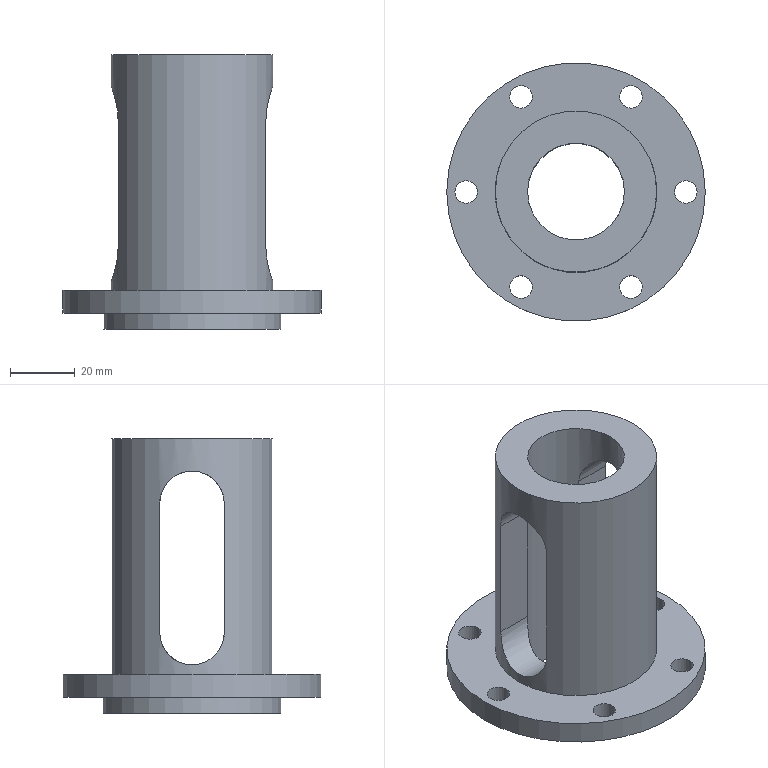Part | NX | 1 solid | 22 faces | box 80 x 80 x 85 mm | volume 105355 mm3 | cylinder 14 | plane 8 | commonest cylinder face diameters 7 x6 20 x4 30 x1 50 x1 55 x1 80 x1
STEP:
#1=CARTESIAN_POINT('',(-18.75,-32.476,12.));
#2=VERTEX_POINT('',#1);
#3=CARTESIAN_POINT('',(-17.,-29.445,12.));
#4=DIRECTION('',(0.,0.,1.));
#5=DIRECTION('',(-0.5,-0.866,0.));
#6=AXIS2_PLACEMENT_3D('',#3,#4,#5);
#7=CIRCLE('',#6,3.5);
#8=EDGE_CURVE('',#2,#2,#7,.T.);
#9=ORIENTED_EDGE('',*,*,#8,.T.);
#10=EDGE_LOOP('',(#9));
#11=FACE_BOUND('',#10,.T.);
#12=CARTESIAN_POINT('',(-18.75,-32.476,5.));
#13=VERTEX_POINT('',#12);
#14=CARTESIAN_POINT('',(-17.,-29.445,5.));
#15=DIRECTION('',(0.,0.,1.));
#16=DIRECTION('',(-0.5,-0.866,0.));
#17=AXIS2_PLACEMENT_3D('',#14,#15,#16);
#18=CIRCLE('',#17,3.5);
#19=EDGE_CURVE('',#13,#13,#18,.T.);
#20=ORIENTED_EDGE('',*,*,#19,.F.);
#21=EDGE_LOOP('',(#20));
#22=FACE_BOUND('',#21,.T.);
#23=CARTESIAN_POINT('',(-17.,-29.445,12.));
#24=DIRECTION('',(0.,0.,-1.));
#25=DIRECTION('',(-1.,0.,0.));
#26=AXIS2_PLACEMENT_3D('',#23,#24,#25);
#27=CYLINDRICAL_SURFACE('',#26,3.5);
#28=ADVANCED_FACE('',(#11,#22),#27,.F.);
#29=CARTESIAN_POINT('',(-18.75,32.476,12.));
#30=VERTEX_POINT('',#29);
#31=CARTESIAN_POINT('',(-17.,29.445,12.));
#32=DIRECTION('',(0.,0.,1.));
#33=DIRECTION('',(-0.5,0.866,0.));
#34=AXIS2_PLACEMENT_3D('',#31,#32,#33);
#35=CIRCLE('',#34,3.5);
#36=EDGE_CURVE('',#30,#30,#35,.T.);
#37=ORIENTED_EDGE('',*,*,#36,.T.);
#38=EDGE_LOOP('',(#37));
#39=FACE_BOUND('',#38,.T.);
#40=CARTESIAN_POINT('',(-18.75,32.476,5.));
#41=VERTEX_POINT('',#40);
#42=CARTESIAN_POINT('',(-17.,29.445,5.));
#43=DIRECTION('',(0.,0.,1.));
#44=DIRECTION('',(-0.5,0.866,0.));
#45=AXIS2_PLACEMENT_3D('',#42,#43,#44);
#46=CIRCLE('',#45,3.5);
#47=EDGE_CURVE('',#41,#41,#46,.T.);
#48=ORIENTED_EDGE('',*,*,#47,.F.);
#49=EDGE_LOOP('',(#48));
#50=FACE_BOUND('',#49,.T.);
#51=CARTESIAN_POINT('',(-17.,29.445,12.));
#52=DIRECTION('',(0.,0.,-1.));
#53=DIRECTION('',(-1.,0.,0.));
#54=AXIS2_PLACEMENT_3D('',#51,#52,#53);
#55=CYLINDRICAL_SURFACE('',#54,3.5);
#56=ADVANCED_FACE('',(#39,#50),#55,.F.);
#57=CARTESIAN_POINT('',(18.75,-32.476,12.));
#58=VERTEX_POINT('',#57);
#59=CARTESIAN_POINT('',(17.,-29.445,12.));
#60=DIRECTION('',(0.,0.,1.));
#61=DIRECTION('',(0.5,-0.866,0.));
#62=AXIS2_PLACEMENT_3D('',#59,#60,#61);
#63=CIRCLE('',#62,3.5);
#64=EDGE_CURVE('',#58,#58,#63,.T.);
#65=ORIENTED_EDGE('',*,*,#64,.T.);
#66=EDGE_LOOP('',(#65));
#67=FACE_BOUND('',#66,.T.);
#68=CARTESIAN_POINT('',(18.75,-32.476,5.));
#69=VERTEX_POINT('',#68);
#70=CARTESIAN_POINT('',(17.,-29.445,5.));
#71=DIRECTION('',(0.,0.,1.));
#72=DIRECTION('',(0.5,-0.866,0.));
#73=AXIS2_PLACEMENT_3D('',#70,#71,#72);
#74=CIRCLE('',#73,3.5);
#75=EDGE_CURVE('',#69,#69,#74,.T.);
#76=ORIENTED_EDGE('',*,*,#75,.F.);
#77=EDGE_LOOP('',(#76));
#78=FACE_BOUND('',#77,.T.);
#79=CARTESIAN_POINT('',(17.,-29.445,12.));
#80=DIRECTION('',(0.,0.,-1.));
#81=DIRECTION('',(-1.,0.,0.));
#82=AXIS2_PLACEMENT_3D('',#79,#80,#81);
#83=CYLINDRICAL_SURFACE('',#82,3.5);
#84=ADVANCED_FACE('',(#67,#78),#83,.F.);
#85=CARTESIAN_POINT('',(18.75,32.476,12.));
#86=VERTEX_POINT('',#85);
#87=CARTESIAN_POINT('',(17.,29.445,12.));
#88=DIRECTION('',(0.,0.,1.));
#89=DIRECTION('',(0.5,0.866,0.));
#90=AXIS2_PLACEMENT_3D('',#87,#88,#89);
#91=CIRCLE('',#90,3.5);
#92=EDGE_CURVE('',#86,#86,#91,.T.);
#93=ORIENTED_EDGE('',*,*,#92,.T.);
#94=EDGE_LOOP('',(#93));
#95=FACE_BOUND('',#94,.T.);
#96=CARTESIAN_POINT('',(18.75,32.476,5.));
#97=VERTEX_POINT('',#96);
#98=CARTESIAN_POINT('',(17.,29.445,5.));
#99=DIRECTION('',(0.,0.,1.));
#100=DIRECTION('',(0.5,0.866,0.));
#101=AXIS2_PLACEMENT_3D('',#98,#99,#100);
#102=CIRCLE('',#101,3.5);
#103=EDGE_CURVE('',#97,#97,#102,.T.);
#104=ORIENTED_EDGE('',*,*,#103,.F.);
#105=EDGE_LOOP('',(#104));
#106=FACE_BOUND('',#105,.T.);
#107=CARTESIAN_POINT('',(17.,29.445,12.));
#108=DIRECTION('',(0.,0.,-1.));
#109=DIRECTION('',(-1.,0.,0.));
#110=AXIS2_PLACEMENT_3D('',#107,#108,#109);
#111=CYLINDRICAL_SURFACE('',#110,3.5);
#112=ADVANCED_FACE('',(#95,#106),#111,.F.);
#113=CARTESIAN_POINT('',(37.5,0.,12.));
#114=VERTEX_POINT('',#113);
#115=CARTESIAN_POINT('',(34.,0.,12.));
#116=DIRECTION('',(0.,0.,1.));
#117=DIRECTION('',(1.,0.,0.));
#118=AXIS2_PLACEMENT_3D('',#115,#116,#117);
#119=CIRCLE('',#118,3.5);
#120=EDGE_CURVE('',#114,#114,#119,.T.);
#121=ORIENTED_EDGE('',*,*,#120,.T.);
#122=EDGE_LOOP('',(#121));
#123=FACE_BOUND('',#122,.T.);
#124=CARTESIAN_POINT('',(37.5,0.,5.));
#125=VERTEX_POINT('',#124);
#126=CARTESIAN_POINT('',(34.,0.,5.));
#127=DIRECTION('',(0.,0.,1.));
#128=DIRECTION('',(1.,0.,0.));
#129=AXIS2_PLACEMENT_3D('',#126,#127,#128);
#130=CIRCLE('',#129,3.5);
#131=EDGE_CURVE('',#125,#125,#130,.T.);
#132=ORIENTED_EDGE('',*,*,#131,.F.);
#133=EDGE_LOOP('',(#132));
#134=FACE_BOUND('',#133,.T.);
#135=CARTESIAN_POINT('',(34.,0.,12.));
#136=DIRECTION('',(0.,0.,-1.));
#137=DIRECTION('',(-1.,0.,0.));
#138=AXIS2_PLACEMENT_3D('',#135,#136,#137);
#139=CYLINDRICAL_SURFACE('',#138,3.5);
#140=ADVANCED_FACE('',(#123,#134),#139,.F.);
#141=CARTESIAN_POINT('',(40.,0.,12.));
#142=VERTEX_POINT('',#141);
#143=CARTESIAN_POINT('',(0.,0.,12.));
#144=DIRECTION('',(0.,0.,1.));
#145=DIRECTION('',(1.,0.,0.));
#146=AXIS2_PLACEMENT_3D('',#143,#144,#145);
#147=CIRCLE('',#146,40.);
#148=EDGE_CURVE('',#142,#142,#147,.T.);
#149=ORIENTED_EDGE('',*,*,#148,.F.);
#150=EDGE_LOOP('',(#149));
#151=FACE_BOUND('',#150,.T.);
#152=CARTESIAN_POINT('',(40.,0.,5.));
#153=VERTEX_POINT('',#152);
#154=CARTESIAN_POINT('',(0.,0.,5.));
#155=DIRECTION('',(0.,0.,-1.));
#156=DIRECTION('',(1.,0.,0.));
#157=AXIS2_PLACEMENT_3D('',#154,#155,#156);
#158=CIRCLE('',#157,40.);
#159=EDGE_CURVE('',#153,#153,#158,.T.);
#160=ORIENTED_EDGE('',*,*,#159,.F.);
#161=EDGE_LOOP('',(#160));
#162=FACE_BOUND('',#161,.T.);
#163=CARTESIAN_POINT('',(0.,0.,12.));
#164=DIRECTION('',(0.,0.,-1.));
#165=DIRECTION('',(-1.,0.,0.));
#166=AXIS2_PLACEMENT_3D('',#163,#164,#165);
#167=CYLINDRICAL_SURFACE('',#166,40.);
#168=ADVANCED_FACE('',(#151,#162),#167,.T.);
#169=CARTESIAN_POINT('',(-37.5,0.,12.));
#170=VERTEX_POINT('',#169);
#171=CARTESIAN_POINT('',(-34.,0.,12.));
#172=DIRECTION('',(0.,0.,1.));
#173=DIRECTION('',(-1.,0.,0.));
#174=AXIS2_PLACEMENT_3D('',#171,#172,#173);
#175=CIRCLE('',#174,3.5);
#176=EDGE_CURVE('',#170,#170,#175,.T.);
#177=ORIENTED_EDGE('',*,*,#176,.T.);
#178=EDGE_LOOP('',(#177));
#179=FACE_BOUND('',#178,.T.);
#180=CARTESIAN_POINT('',(-37.5,0.,5.));
#181=VERTEX_POINT('',#180);
#182=CARTESIAN_POINT('',(-34.,0.,5.));
#183=DIRECTION('',(0.,0.,1.));
#184=DIRECTION('',(-1.,0.,0.));
#185=AXIS2_PLACEMENT_3D('',#182,#183,#184);
#186=CIRCLE('',#185,3.5);
#187=EDGE_CURVE('',#181,#181,#186,.T.);
#188=ORIENTED_EDGE('',*,*,#187,.F.);
#189=EDGE_LOOP('',(#188));
#190=FACE_BOUND('',#189,.T.);
#191=CARTESIAN_POINT('',(-34.,0.,12.));
#192=DIRECTION('',(0.,0.,-1.));
#193=DIRECTION('',(-1.,0.,0.));
#194=AXIS2_PLACEMENT_3D('',#191,#192,#193);
#195=CYLINDRICAL_SURFACE('',#194,3.5);
#196=ADVANCED_FACE('',(#179,#190),#195,.F.);
#197=CARTESIAN_POINT('',(22.913,10.,65.));
#198=VERTEX_POINT('',#197);
#199=CARTESIAN_POINT('',(22.913,-10.,65.));
#200=VERTEX_POINT('',#199);
#201=CARTESIAN_POINT('',(22.913,10.,65.));
#202=CARTESIAN_POINT('',(22.913,10.,67.672));
#203=CARTESIAN_POINT('',(23.712,8.35,71.514));
#204=CARTESIAN_POINT('',(24.779,3.969,74.459));
#205=CARTESIAN_POINT('',(25.11,0.01559,75.268));
#206=CARTESIAN_POINT('',(24.782,-3.957,74.467));
#207=CARTESIAN_POINT('',(23.711,-8.353,71.514));
#208=CARTESIAN_POINT('',(22.913,-10.,67.673));
#209=CARTESIAN_POINT('',(22.913,-10.,65.));
#210=B_SPLINE_CURVE_WITH_KNOTS('',3,(#201,#202,#203,#204,#205,#206,#207,#208,#209),.UNSPECIFIED.,.F.,.F.,(4,1,1,1,1,1,4),(0.,0.007896,0.01184,0.01579,0.01974,0.02369,0.03158),.UNSPECIFIED.);
#211=EDGE_CURVE('',#198,#200,#210,.T.);
#212=ORIENTED_EDGE('',*,*,#211,.F.);
#213=CARTESIAN_POINT('',(22.913,10.,25.));
#214=VERTEX_POINT('',#213);
#215=CARTESIAN_POINT('',(22.913,10.,85.));
#216=DIRECTION('',(0.,0.,-1.));
#217=VECTOR('',#216,1000.);
#218=LINE('',#215,#217);
#219=EDGE_CURVE('',#214,#198,#218,.F.);
#220=ORIENTED_EDGE('',*,*,#219,.F.);
#221=CARTESIAN_POINT('',(22.913,-10.,25.));
#222=VERTEX_POINT('',#221);
#223=CARTESIAN_POINT('',(22.913,-10.,25.));
#224=CARTESIAN_POINT('',(22.913,-10.,22.328));
#225=CARTESIAN_POINT('',(23.712,-8.35,18.486));
#226=CARTESIAN_POINT('',(24.779,-3.969,15.541));
#227=CARTESIAN_POINT('',(25.11,-0.01559,14.732));
#228=CARTESIAN_POINT('',(24.782,3.957,15.533));
#229=CARTESIAN_POINT('',(23.711,8.353,18.486));
#230=CARTESIAN_POINT('',(22.913,10.,22.327));
#231=CARTESIAN_POINT('',(22.913,10.,25.));
#232=B_SPLINE_CURVE_WITH_KNOTS('',3,(#223,#224,#225,#226,#227,#228,#229,#230,#231),.UNSPECIFIED.,.F.,.F.,(4,1,1,1,1,1,4),(0.,0.007896,0.01184,0.01579,0.01974,0.02369,0.03158),.UNSPECIFIED.);
#233=EDGE_CURVE('',#222,#214,#232,.T.);
#234=ORIENTED_EDGE('',*,*,#233,.F.);
#235=CARTESIAN_POINT('',(22.913,-10.,85.));
#236=DIRECTION('',(0.,0.,-1.));
#237=VECTOR('',#236,1000.);
#238=LINE('',#235,#237);
#239=EDGE_CURVE('',#200,#222,#238,.T.);
#240=ORIENTED_EDGE('',*,*,#239,.F.);
#241=EDGE_LOOP('',(#212,#220,#234,#240));
#242=FACE_BOUND('',#241,.T.);
#243=CARTESIAN_POINT('',(25.,0.,85.));
#244=VERTEX_POINT('',#243);
#245=CARTESIAN_POINT('',(0.,0.,85.));
#246=DIRECTION('',(0.,0.,1.));
#247=DIRECTION('',(1.,0.,0.));
#248=AXIS2_PLACEMENT_3D('',#245,#246,#247);
#249=CIRCLE('',#248,25.);
#250=EDGE_CURVE('',#244,#244,#249,.T.);
#251=ORIENTED_EDGE('',*,*,#250,.F.);
#252=EDGE_LOOP('',(#251));
#253=FACE_BOUND('',#252,.T.);
#254=CARTESIAN_POINT('',(25.,0.,12.));
#255=VERTEX_POINT('',#254);
#256=CARTESIAN_POINT('',(0.,0.,12.));
#257=DIRECTION('',(0.,0.,1.));
#258=DIRECTION('',(1.,0.,0.));
#259=AXIS2_PLACEMENT_3D('',#256,#257,#258);
#260=CIRCLE('',#259,25.);
#261=EDGE_CURVE('',#255,#255,#260,.T.);
#262=ORIENTED_EDGE('',*,*,#261,.T.);
#263=EDGE_LOOP('',(#262));
#264=FACE_BOUND('',#263,.T.);
#265=CARTESIAN_POINT('',(-22.913,10.,65.));
#266=VERTEX_POINT('',#265);
#267=CARTESIAN_POINT('',(-22.913,10.,25.));
#268=VERTEX_POINT('',#267);
#269=CARTESIAN_POINT('',(-22.913,10.,85.));
#270=DIRECTION('',(0.,0.,-1.));
#271=VECTOR('',#270,1000.);
#272=LINE('',#269,#271);
#273=EDGE_CURVE('',#266,#268,#272,.T.);
#274=ORIENTED_EDGE('',*,*,#273,.F.);
#275=CARTESIAN_POINT('',(-22.913,-10.,65.));
#276=VERTEX_POINT('',#275);
#277=CARTESIAN_POINT('',(-22.913,-10.,65.));
#278=CARTESIAN_POINT('',(-22.913,-10.,67.672));
#279=CARTESIAN_POINT('',(-23.712,-8.35,71.514));
#280=CARTESIAN_POINT('',(-24.779,-3.969,74.459));
#281=CARTESIAN_POINT('',(-25.11,-0.01559,75.268));
#282=CARTESIAN_POINT('',(-24.782,3.957,74.467));
#283=CARTESIAN_POINT('',(-23.711,8.353,71.514));
#284=CARTESIAN_POINT('',(-22.913,10.,67.673));
#285=CARTESIAN_POINT('',(-22.913,10.,65.));
#286=B_SPLINE_CURVE_WITH_KNOTS('',3,(#277,#278,#279,#280,#281,#282,#283,#284,#285),.UNSPECIFIED.,.F.,.F.,(4,1,1,1,1,1,4),(0.,0.007896,0.01184,0.01579,0.01974,0.02369,0.03158),.UNSPECIFIED.);
#287=EDGE_CURVE('',#276,#266,#286,.T.);
#288=ORIENTED_EDGE('',*,*,#287,.F.);
#289=CARTESIAN_POINT('',(-22.913,-10.,25.));
#290=VERTEX_POINT('',#289);
#291=CARTESIAN_POINT('',(-22.913,-10.,85.));
#292=DIRECTION('',(0.,0.,-1.));
#293=VECTOR('',#292,1000.);
#294=LINE('',#291,#293);
#295=EDGE_CURVE('',#290,#276,#294,.F.);
#296=ORIENTED_EDGE('',*,*,#295,.F.);
#297=CARTESIAN_POINT('',(-22.913,10.,25.));
#298=CARTESIAN_POINT('',(-22.913,10.,22.328));
#299=CARTESIAN_POINT('',(-23.712,8.35,18.486));
#300=CARTESIAN_POINT('',(-24.779,3.969,15.541));
#301=CARTESIAN_POINT('',(-25.11,0.01559,14.732));
#302=CARTESIAN_POINT('',(-24.782,-3.957,15.533));
#303=CARTESIAN_POINT('',(-23.711,-8.353,18.486));
#304=CARTESIAN_POINT('',(-22.913,-10.,22.327));
#305=CARTESIAN_POINT('',(-22.913,-10.,25.));
#306=B_SPLINE_CURVE_WITH_KNOTS('',3,(#297,#298,#299,#300,#301,#302,#303,#304,#305),.UNSPECIFIED.,.F.,.F.,(4,1,1,1,1,1,4),(0.,0.007896,0.01184,0.01579,0.01974,0.02369,0.03158),.UNSPECIFIED.);
#307=EDGE_CURVE('',#268,#290,#306,.T.);
#308=ORIENTED_EDGE('',*,*,#307,.F.);
#309=EDGE_LOOP('',(#274,#288,#296,#308));
#310=FACE_BOUND('',#309,.T.);
#311=CARTESIAN_POINT('',(0.,0.,85.));
#312=DIRECTION('',(0.,0.,-1.));
#313=DIRECTION('',(-1.,0.,0.));
#314=AXIS2_PLACEMENT_3D('',#311,#312,#313);
#315=CYLINDRICAL_SURFACE('',#314,25.);
#316=ADVANCED_FACE('',(#242,#253,#264,#310),#315,.T.);
#317=CARTESIAN_POINT('',(15.,0.,85.));
#318=VERTEX_POINT('',#317);
#319=CARTESIAN_POINT('',(0.,0.,85.));
#320=DIRECTION('',(0.,0.,1.));
#321=DIRECTION('',(1.,0.,0.));
#322=AXIS2_PLACEMENT_3D('',#319,#320,#321);
#323=CIRCLE('',#322,15.);
#324=EDGE_CURVE('',#318,#318,#323,.T.);
#325=ORIENTED_EDGE('',*,*,#324,.T.);
#326=EDGE_LOOP('',(#325));
#327=FACE_BOUND('',#326,.T.);
#328=CARTESIAN_POINT('',(15.,0.,0.));
#329=VERTEX_POINT('',#328);
#330=CARTESIAN_POINT('',(0.,0.,0.));
#331=DIRECTION('',(0.,0.,1.));
#332=DIRECTION('',(1.,0.,0.));
#333=AXIS2_PLACEMENT_3D('',#330,#331,#332);
#334=CIRCLE('',#333,15.);
#335=EDGE_CURVE('',#329,#329,#334,.T.);
#336=ORIENTED_EDGE('',*,*,#335,.F.);
#337=EDGE_LOOP('',(#336));
#338=FACE_BOUND('',#337,.T.);
#339=CARTESIAN_POINT('',(11.18,-10.,25.));
#340=VERTEX_POINT('',#339);
#341=CARTESIAN_POINT('',(11.18,10.,25.));
#342=VERTEX_POINT('',#341);
#343=CARTESIAN_POINT('',(11.18,-10.,25.));
#344=CARTESIAN_POINT('',(11.18,-10.,23.63));
#345=CARTESIAN_POINT('',(11.718,-9.43,20.978));
#346=CARTESIAN_POINT('',(13.243,-7.268,17.79));
#347=CARTESIAN_POINT('',(14.604,-4.071,15.581));
#348=CARTESIAN_POINT('',(15.195,-0.03414,14.714));
#349=CARTESIAN_POINT('',(14.616,4.041,15.562));
#350=CARTESIAN_POINT('',(13.247,7.261,17.785));
#351=CARTESIAN_POINT('',(11.727,9.419,20.951));
#352=CARTESIAN_POINT('',(11.18,10.,23.627));
#353=CARTESIAN_POINT('',(11.18,10.,25.));
#354=B_SPLINE_CURVE_WITH_KNOTS('',3,(#343,#344,#345,#346,#347,#348,#349,#350,#351,#352,#353),.UNSPECIFIED.,.F.,.F.,(4,1,1,1,1,1,1,1,4),(0.,0.004037,0.008074,0.01211,0.01615,0.02018,0.02422,0.02826,0.0323),.UNSPECIFIED.);
#355=EDGE_CURVE('',#340,#342,#354,.T.);
#356=ORIENTED_EDGE('',*,*,#355,.T.);
#357=CARTESIAN_POINT('',(11.18,10.,65.));
#358=VERTEX_POINT('',#357);
#359=CARTESIAN_POINT('',(11.18,10.,85.));
#360=DIRECTION('',(0.,0.,-1.));
#361=VECTOR('',#360,1000.);
#362=LINE('',#359,#361);
#363=EDGE_CURVE('',#342,#358,#362,.F.);
#364=ORIENTED_EDGE('',*,*,#363,.T.);
#365=CARTESIAN_POINT('',(11.18,-10.,65.));
#366=VERTEX_POINT('',#365);
#367=CARTESIAN_POINT('',(11.18,10.,65.));
#368=CARTESIAN_POINT('',(11.18,10.,66.37));
#369=CARTESIAN_POINT('',(11.718,9.43,69.022));
#370=CARTESIAN_POINT('',(13.243,7.268,72.21));
#371=CARTESIAN_POINT('',(14.604,4.071,74.419));
#372=CARTESIAN_POINT('',(15.195,0.03414,75.286));
#373=CARTESIAN_POINT('',(14.616,-4.041,74.438));
#374=CARTESIAN_POINT('',(13.247,-7.261,72.215));
#375=CARTESIAN_POINT('',(11.727,-9.419,69.049));
#376=CARTESIAN_POINT('',(11.18,-10.,66.373));
#377=CARTESIAN_POINT('',(11.18,-10.,65.));
#378=B_SPLINE_CURVE_WITH_KNOTS('',3,(#367,#368,#369,#370,#371,#372,#373,#374,#375,#376,#377),.UNSPECIFIED.,.F.,.F.,(4,1,1,1,1,1,1,1,4),(0.,0.004037,0.008074,0.01211,0.01615,0.02018,0.02422,0.02826,0.0323),.UNSPECIFIED.);
#379=EDGE_CURVE('',#358,#366,#378,.T.);
#380=ORIENTED_EDGE('',*,*,#379,.T.);
#381=CARTESIAN_POINT('',(11.18,-10.,85.));
#382=DIRECTION('',(0.,0.,-1.));
#383=VECTOR('',#382,1000.);
#384=LINE('',#381,#383);
#385=EDGE_CURVE('',#366,#340,#384,.T.);
#386=ORIENTED_EDGE('',*,*,#385,.T.);
#387=EDGE_LOOP('',(#356,#364,#380,#386));
#388=FACE_BOUND('',#387,.T.);
#389=CARTESIAN_POINT('',(-11.18,-10.,65.));
#390=VERTEX_POINT('',#389);
#391=CARTESIAN_POINT('',(-11.18,10.,65.));
#392=VERTEX_POINT('',#391);
#393=CARTESIAN_POINT('',(-11.18,-10.,65.));
#394=CARTESIAN_POINT('',(-11.18,-10.,66.37));
#395=CARTESIAN_POINT('',(-11.718,-9.43,69.022));
#396=CARTESIAN_POINT('',(-13.243,-7.268,72.21));
#397=CARTESIAN_POINT('',(-14.604,-4.071,74.419));
#398=CARTESIAN_POINT('',(-15.195,-0.03414,75.286));
#399=CARTESIAN_POINT('',(-14.616,4.041,74.438));
#400=CARTESIAN_POINT('',(-13.247,7.261,72.215));
#401=CARTESIAN_POINT('',(-11.727,9.419,69.049));
#402=CARTESIAN_POINT('',(-11.18,10.,66.373));
#403=CARTESIAN_POINT('',(-11.18,10.,65.));
#404=B_SPLINE_CURVE_WITH_KNOTS('',3,(#393,#394,#395,#396,#397,#398,#399,#400,#401,#402,#403),.UNSPECIFIED.,.F.,.F.,(4,1,1,1,1,1,1,1,4),(0.,0.004037,0.008074,0.01211,0.01615,0.02018,0.02422,0.02826,0.0323),.UNSPECIFIED.);
#405=EDGE_CURVE('',#390,#392,#404,.T.);
#406=ORIENTED_EDGE('',*,*,#405,.T.);
#407=CARTESIAN_POINT('',(-11.18,10.,25.));
#408=VERTEX_POINT('',#407);
#409=CARTESIAN_POINT('',(-11.18,10.,85.));
#410=DIRECTION('',(0.,0.,-1.));
#411=VECTOR('',#410,1000.);
#412=LINE('',#409,#411);
#413=EDGE_CURVE('',#392,#408,#412,.T.);
#414=ORIENTED_EDGE('',*,*,#413,.T.);
#415=CARTESIAN_POINT('',(-11.18,-10.,25.));
#416=VERTEX_POINT('',#415);
#417=CARTESIAN_POINT('',(-11.18,10.,25.));
#418=CARTESIAN_POINT('',(-11.18,10.,23.63));
#419=CARTESIAN_POINT('',(-11.718,9.43,20.978));
#420=CARTESIAN_POINT('',(-13.243,7.268,17.79));
#421=CARTESIAN_POINT('',(-14.604,4.071,15.581));
#422=CARTESIAN_POINT('',(-15.195,0.03414,14.714));
#423=CARTESIAN_POINT('',(-14.616,-4.041,15.562));
#424=CARTESIAN_POINT('',(-13.247,-7.261,17.785));
#425=CARTESIAN_POINT('',(-11.727,-9.419,20.951));
#426=CARTESIAN_POINT('',(-11.18,-10.,23.627));
#427=CARTESIAN_POINT('',(-11.18,-10.,25.));
#428=B_SPLINE_CURVE_WITH_KNOTS('',3,(#417,#418,#419,#420,#421,#422,#423,#424,#425,#426,#427),.UNSPECIFIED.,.F.,.F.,(4,1,1,1,1,1,1,1,4),(0.,0.004037,0.008074,0.01211,0.01615,0.02018,0.02422,0.02826,0.0323),.UNSPECIFIED.);
#429=EDGE_CURVE('',#408,#416,#428,.T.);
#430=ORIENTED_EDGE('',*,*,#429,.T.);
#431=CARTESIAN_POINT('',(-11.18,-10.,85.));
#432=DIRECTION('',(0.,0.,-1.));
#433=VECTOR('',#432,1000.);
#434=LINE('',#431,#433);
#435=EDGE_CURVE('',#416,#390,#434,.F.);
#436=ORIENTED_EDGE('',*,*,#435,.T.);
#437=EDGE_LOOP('',(#406,#414,#430,#436));
#438=FACE_BOUND('',#437,.T.);
#439=CARTESIAN_POINT('',(0.,0.,85.));
#440=DIRECTION('',(0.,0.,-1.));
#441=DIRECTION('',(-1.,0.,0.));
#442=AXIS2_PLACEMENT_3D('',#439,#440,#441);
#443=CYLINDRICAL_SURFACE('',#442,15.);
#444=ADVANCED_FACE('',(#327,#338,#388,#438),#443,.F.);
#445=ORIENTED_EDGE('',*,*,#250,.T.);
#446=EDGE_LOOP('',(#445));
#447=FACE_BOUND('',#446,.T.);
#448=ORIENTED_EDGE('',*,*,#324,.F.);
#449=EDGE_LOOP('',(#448));
#450=FACE_BOUND('',#449,.T.);
#451=CARTESIAN_POINT('',(0.,0.,85.));
#452=DIRECTION('',(0.,0.,1.));
#453=DIRECTION('',(1.,0.,0.));
#454=AXIS2_PLACEMENT_3D('',#451,#452,#453);
#455=PLANE('',#454);
#456=ADVANCED_FACE('',(#447,#450),#455,.T.);
#457=CARTESIAN_POINT('',(27.5,0.,0.));
#458=VERTEX_POINT('',#457);
#459=CARTESIAN_POINT('',(0.,0.,0.));
#460=DIRECTION('',(0.,0.,1.));
#461=DIRECTION('',(1.,0.,0.));
#462=AXIS2_PLACEMENT_3D('',#459,#460,#461);
#463=CIRCLE('',#462,27.5);
#464=EDGE_CURVE('',#458,#458,#463,.T.);
#465=ORIENTED_EDGE('',*,*,#464,.F.);
#466=EDGE_LOOP('',(#465));
#467=FACE_BOUND('',#466,.T.);
#468=ORIENTED_EDGE('',*,*,#335,.T.);
#469=EDGE_LOOP('',(#468));
#470=FACE_BOUND('',#469,.T.);
#471=CARTESIAN_POINT('',(0.,0.,0.));
#472=DIRECTION('',(0.,0.,1.));
#473=DIRECTION('',(1.,0.,0.));
#474=AXIS2_PLACEMENT_3D('',#471,#472,#473);
#475=PLANE('',#474);
#476=ADVANCED_FACE('',(#467,#470),#475,.F.);
#477=ORIENTED_EDGE('',*,*,#148,.T.);
#478=EDGE_LOOP('',(#477));
#479=FACE_BOUND('',#478,.T.);
#480=ORIENTED_EDGE('',*,*,#120,.F.);
#481=EDGE_LOOP('',(#480));
#482=FACE_BOUND('',#481,.T.);
#483=ORIENTED_EDGE('',*,*,#92,.F.);
#484=EDGE_LOOP('',(#483));
#485=FACE_BOUND('',#484,.T.);
#486=ORIENTED_EDGE('',*,*,#64,.F.);
#487=EDGE_LOOP('',(#486));
#488=FACE_BOUND('',#487,.T.);
#489=ORIENTED_EDGE('',*,*,#36,.F.);
#490=EDGE_LOOP('',(#489));
#491=FACE_BOUND('',#490,.T.);
#492=ORIENTED_EDGE('',*,*,#8,.F.);
#493=EDGE_LOOP('',(#492));
#494=FACE_BOUND('',#493,.T.);
#495=ORIENTED_EDGE('',*,*,#261,.F.);
#496=EDGE_LOOP('',(#495));
#497=FACE_BOUND('',#496,.T.);
#498=ORIENTED_EDGE('',*,*,#176,.F.);
#499=EDGE_LOOP('',(#498));
#500=FACE_BOUND('',#499,.T.);
#501=CARTESIAN_POINT('',(17.,0.,12.));
#502=DIRECTION('',(0.,0.,1.));
#503=DIRECTION('',(1.,0.,0.));
#504=AXIS2_PLACEMENT_3D('',#501,#502,#503);
#505=PLANE('',#504);
#506=ADVANCED_FACE('',(#479,#482,#485,#488,#491,#494,#497,#500),#505,.T.);
#507=ORIENTED_EDGE('',*,*,#211,.T.);
#508=CARTESIAN_POINT('',(-75.,-10.,65.));
#509=DIRECTION('',(1.,0.,0.));
#510=VECTOR('',#509,1000.);
#511=LINE('',#508,#510);
#512=EDGE_CURVE('',#200,#366,#511,.F.);
#513=ORIENTED_EDGE('',*,*,#512,.T.);
#514=ORIENTED_EDGE('',*,*,#379,.F.);
#515=CARTESIAN_POINT('',(-75.,10.,65.));
#516=DIRECTION('',(1.,0.,0.));
#517=VECTOR('',#516,1000.);
#518=LINE('',#515,#517);
#519=EDGE_CURVE('',#198,#358,#518,.F.);
#520=ORIENTED_EDGE('',*,*,#519,.F.);
#521=EDGE_LOOP('',(#507,#513,#514,#520));
#522=FACE_BOUND('',#521,.T.);
#523=CARTESIAN_POINT('',(-75.,0.,65.));
#524=DIRECTION('',(1.,0.,0.));
#525=DIRECTION('',(0.,0.,-1.));
#526=AXIS2_PLACEMENT_3D('',#523,#524,#525);
#527=CYLINDRICAL_SURFACE('',#526,10.);
#528=ADVANCED_FACE('',(#522),#527,.F.);
#529=ORIENTED_EDGE('',*,*,#239,.T.);
#530=CARTESIAN_POINT('',(-75.,-10.,25.));
#531=DIRECTION('',(1.,0.,0.));
#532=VECTOR('',#531,1000.);
#533=LINE('',#530,#532);
#534=EDGE_CURVE('',#222,#340,#533,.F.);
#535=ORIENTED_EDGE('',*,*,#534,.T.);
#536=ORIENTED_EDGE('',*,*,#385,.F.);
#537=ORIENTED_EDGE('',*,*,#512,.F.);
#538=EDGE_LOOP('',(#529,#535,#536,#537));
#539=FACE_BOUND('',#538,.T.);
#540=CARTESIAN_POINT('',(-75.,-10.,25.));
#541=DIRECTION('',(0.,1.,0.));
#542=DIRECTION('',(0.,0.,1.));
#543=AXIS2_PLACEMENT_3D('',#540,#541,#542);
#544=PLANE('',#543);
#545=ADVANCED_FACE('',(#539),#544,.T.);
#546=ORIENTED_EDGE('',*,*,#233,.T.);
#547=CARTESIAN_POINT('',(-75.,10.,25.));
#548=DIRECTION('',(1.,0.,0.));
#549=VECTOR('',#548,1000.);
#550=LINE('',#547,#549);
#551=EDGE_CURVE('',#214,#342,#550,.F.);
#552=ORIENTED_EDGE('',*,*,#551,.T.);
#553=ORIENTED_EDGE('',*,*,#355,.F.);
#554=ORIENTED_EDGE('',*,*,#534,.F.);
#555=EDGE_LOOP('',(#546,#552,#553,#554));
#556=FACE_BOUND('',#555,.T.);
#557=CARTESIAN_POINT('',(-75.,0.,25.));
#558=DIRECTION('',(1.,0.,0.));
#559=DIRECTION('',(0.,0.,-1.));
#560=AXIS2_PLACEMENT_3D('',#557,#558,#559);
#561=CYLINDRICAL_SURFACE('',#560,10.);
#562=ADVANCED_FACE('',(#556),#561,.F.);
#563=ORIENTED_EDGE('',*,*,#219,.T.);
#564=ORIENTED_EDGE('',*,*,#519,.T.);
#565=ORIENTED_EDGE('',*,*,#363,.F.);
#566=ORIENTED_EDGE('',*,*,#551,.F.);
#567=EDGE_LOOP('',(#563,#564,#565,#566));
#568=FACE_BOUND('',#567,.T.);
#569=CARTESIAN_POINT('',(-75.,10.,65.));
#570=DIRECTION('',(0.,-1.,0.));
#571=DIRECTION('',(0.,0.,-1.));
#572=AXIS2_PLACEMENT_3D('',#569,#570,#571);
#573=PLANE('',#572);
#574=ADVANCED_FACE('',(#568),#573,.T.);
#575=ORIENTED_EDGE('',*,*,#273,.T.);
#576=CARTESIAN_POINT('',(-75.,10.,25.));
#577=DIRECTION('',(1.,0.,0.));
#578=VECTOR('',#577,1000.);
#579=LINE('',#576,#578);
#580=EDGE_CURVE('',#408,#268,#579,.F.);
#581=ORIENTED_EDGE('',*,*,#580,.F.);
#582=ORIENTED_EDGE('',*,*,#413,.F.);
#583=CARTESIAN_POINT('',(-75.,10.,65.));
#584=DIRECTION('',(1.,0.,0.));
#585=VECTOR('',#584,1000.);
#586=LINE('',#583,#585);
#587=EDGE_CURVE('',#392,#266,#586,.F.);
#588=ORIENTED_EDGE('',*,*,#587,.T.);
#589=EDGE_LOOP('',(#575,#581,#582,#588));
#590=FACE_BOUND('',#589,.T.);
#591=CARTESIAN_POINT('',(-75.,10.,65.));
#592=DIRECTION('',(0.,-1.,0.));
#593=DIRECTION('',(0.,0.,-1.));
#594=AXIS2_PLACEMENT_3D('',#591,#592,#593);
#595=PLANE('',#594);
#596=ADVANCED_FACE('',(#590),#595,.T.);
#597=ORIENTED_EDGE('',*,*,#307,.T.);
#598=CARTESIAN_POINT('',(-75.,-10.,25.));
#599=DIRECTION('',(1.,0.,0.));
#600=VECTOR('',#599,1000.);
#601=LINE('',#598,#600);
#602=EDGE_CURVE('',#416,#290,#601,.F.);
#603=ORIENTED_EDGE('',*,*,#602,.F.);
#604=ORIENTED_EDGE('',*,*,#429,.F.);
#605=ORIENTED_EDGE('',*,*,#580,.T.);
#606=EDGE_LOOP('',(#597,#603,#604,#605));
#607=FACE_BOUND('',#606,.T.);
#608=CARTESIAN_POINT('',(-75.,0.,25.));
#609=DIRECTION('',(1.,0.,0.));
#610=DIRECTION('',(0.,0.,-1.));
#611=AXIS2_PLACEMENT_3D('',#608,#609,#610);
#612=CYLINDRICAL_SURFACE('',#611,10.);
#613=ADVANCED_FACE('',(#607),#612,.F.);
#614=ORIENTED_EDGE('',*,*,#295,.T.);
#615=CARTESIAN_POINT('',(-75.,-10.,65.));
#616=DIRECTION('',(1.,0.,0.));
#617=VECTOR('',#616,1000.);
#618=LINE('',#615,#617);
#619=EDGE_CURVE('',#390,#276,#618,.F.);
#620=ORIENTED_EDGE('',*,*,#619,.F.);
#621=ORIENTED_EDGE('',*,*,#435,.F.);
#622=ORIENTED_EDGE('',*,*,#602,.T.);
#623=EDGE_LOOP('',(#614,#620,#621,#622));
#624=FACE_BOUND('',#623,.T.);
#625=CARTESIAN_POINT('',(-75.,-10.,25.));
#626=DIRECTION('',(0.,1.,0.));
#627=DIRECTION('',(0.,0.,1.));
#628=AXIS2_PLACEMENT_3D('',#625,#626,#627);
#629=PLANE('',#628);
#630=ADVANCED_FACE('',(#624),#629,.T.);
#631=ORIENTED_EDGE('',*,*,#287,.T.);
#632=ORIENTED_EDGE('',*,*,#587,.F.);
#633=ORIENTED_EDGE('',*,*,#405,.F.);
#634=ORIENTED_EDGE('',*,*,#619,.T.);
#635=EDGE_LOOP('',(#631,#632,#633,#634));
#636=FACE_BOUND('',#635,.T.);
#637=CARTESIAN_POINT('',(-75.,0.,65.));
#638=DIRECTION('',(1.,0.,0.));
#639=DIRECTION('',(0.,0.,-1.));
#640=AXIS2_PLACEMENT_3D('',#637,#638,#639);
#641=CYLINDRICAL_SURFACE('',#640,10.);
#642=ADVANCED_FACE('',(#636),#641,.F.);
#643=CARTESIAN_POINT('',(27.5,0.,5.));
#644=VERTEX_POINT('',#643);
#645=CARTESIAN_POINT('',(0.,0.,5.));
#646=DIRECTION('',(0.,0.,1.));
#647=DIRECTION('',(1.,0.,0.));
#648=AXIS2_PLACEMENT_3D('',#645,#646,#647);
#649=CIRCLE('',#648,27.5);
#650=EDGE_CURVE('',#644,#644,#649,.F.);
#651=ORIENTED_EDGE('',*,*,#650,.T.);
#652=EDGE_LOOP('',(#651));
#653=FACE_BOUND('',#652,.T.);
#654=ORIENTED_EDGE('',*,*,#464,.T.);
#655=EDGE_LOOP('',(#654));
#656=FACE_BOUND('',#655,.T.);
#657=CARTESIAN_POINT('',(0.,0.,5.));
#658=DIRECTION('',(0.,0.,-1.));
#659=DIRECTION('',(-1.,0.,0.));
#660=AXIS2_PLACEMENT_3D('',#657,#658,#659);
#661=CYLINDRICAL_SURFACE('',#660,27.5);
#662=ADVANCED_FACE('',(#653,#656),#661,.T.);
#663=ORIENTED_EDGE('',*,*,#159,.T.);
#664=EDGE_LOOP('',(#663));
#665=FACE_BOUND('',#664,.T.);
#666=ORIENTED_EDGE('',*,*,#131,.T.);
#667=EDGE_LOOP('',(#666));
#668=FACE_BOUND('',#667,.T.);
#669=ORIENTED_EDGE('',*,*,#103,.T.);
#670=EDGE_LOOP('',(#669));
#671=FACE_BOUND('',#670,.T.);
#672=ORIENTED_EDGE('',*,*,#75,.T.);
#673=EDGE_LOOP('',(#672));
#674=FACE_BOUND('',#673,.T.);
#675=ORIENTED_EDGE('',*,*,#47,.T.);
#676=EDGE_LOOP('',(#675));
#677=FACE_BOUND('',#676,.T.);
#678=ORIENTED_EDGE('',*,*,#19,.T.);
#679=EDGE_LOOP('',(#678));
#680=FACE_BOUND('',#679,.T.);
#681=ORIENTED_EDGE('',*,*,#650,.F.);
#682=EDGE_LOOP('',(#681));
#683=FACE_BOUND('',#682,.T.);
#684=ORIENTED_EDGE('',*,*,#187,.T.);
#685=EDGE_LOOP('',(#684));
#686=FACE_BOUND('',#685,.T.);
#687=CARTESIAN_POINT('',(17.,0.,5.));
#688=DIRECTION('',(0.,0.,-1.));
#689=DIRECTION('',(-1.,0.,0.));
#690=AXIS2_PLACEMENT_3D('',#687,#688,#689);
#691=PLANE('',#690);
#692=ADVANCED_FACE('',(#665,#668,#671,#674,#677,#680,#683,#686),#691,.T.);
#693=CLOSED_SHELL('',(#28,#56,#84,#112,#140,#168,#196,#316,#444,#456,#476,#506,#528,#545,#562,#574,#596,#613,#630,#642,#662,#692));
#694=MANIFOLD_SOLID_BREP('',#693);
#695=(LENGTH_UNIT()NAMED_UNIT(*)SI_UNIT(.MILLI.,.METRE.));
#696=UNCERTAINTY_MEASURE_WITH_UNIT(LENGTH_MEASURE(0.0508),#695,'','');
#697=(NAMED_UNIT(*)PLANE_ANGLE_UNIT()SI_UNIT($,.RADIAN.));
#698=(NAMED_UNIT(*)SI_UNIT($,.STERADIAN.)SOLID_ANGLE_UNIT());
#699=(GEOMETRIC_REPRESENTATION_CONTEXT(3)GLOBAL_UNCERTAINTY_ASSIGNED_CONTEXT((#696))GLOBAL_UNIT_ASSIGNED_CONTEXT((#695,#697,#698))REPRESENTATION_CONTEXT('',''));
#700=ADVANCED_BREP_SHAPE_REPRESENTATION('',(#694),#699);